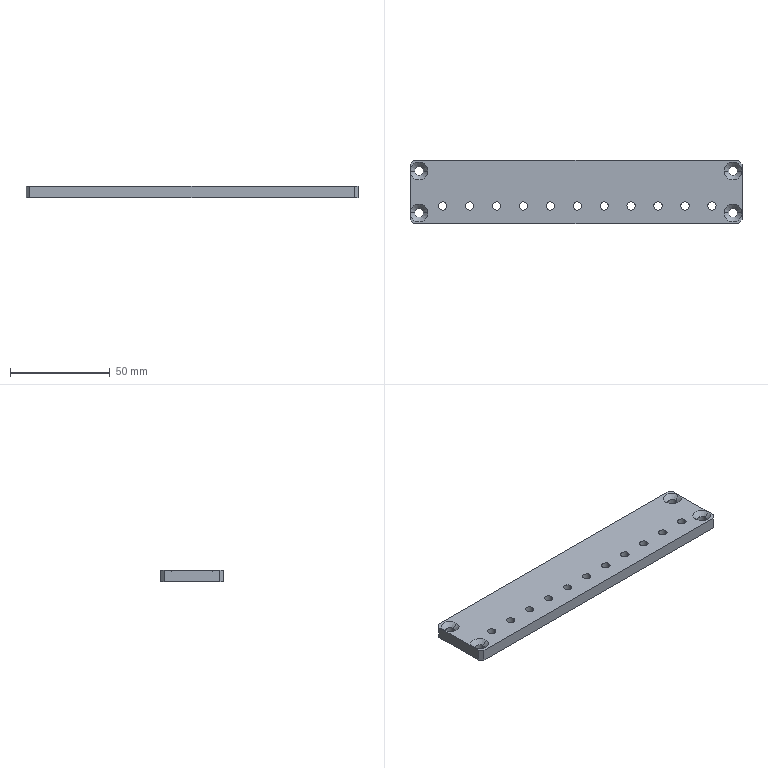Part | STEP file | QA-AD10 | 1 solid | 48 faces | box 166.5 x 32 x 6 mm | volume 30437 mm3 | cylinder 30 | plane 10 | cone 8 | commonest cylinder face diameters 4.2 x22 4.5 x8